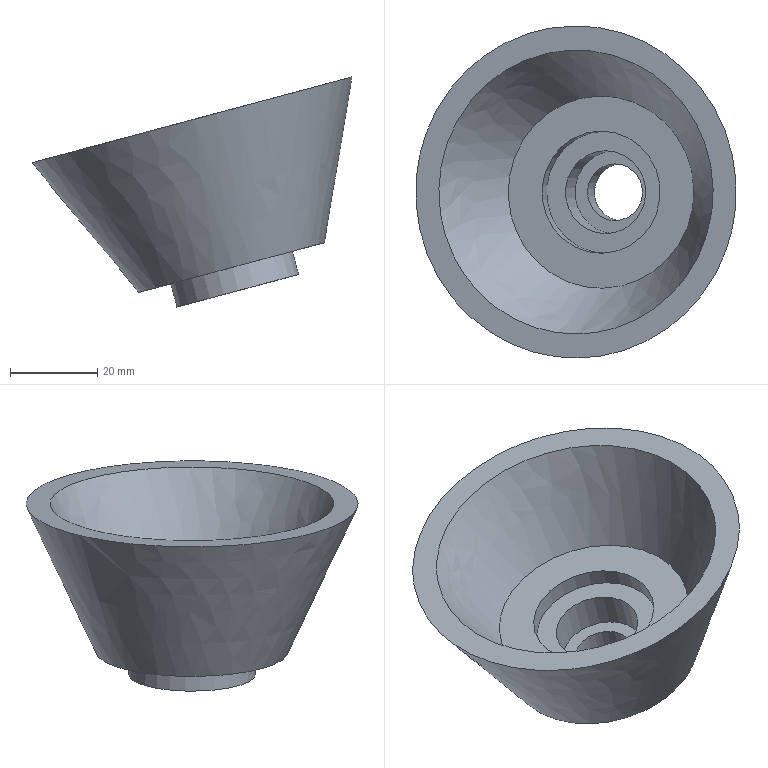Part | NX | features solid 2 | 1 solid | 12 faces | box 73.411 x 76.001 x 52.708 mm | volume 46952 mm3 | plane 6 | cylinder 4 | spline 2 | commonest cylinder face diameters 13 x1 19 x1 28 x1 29 x1